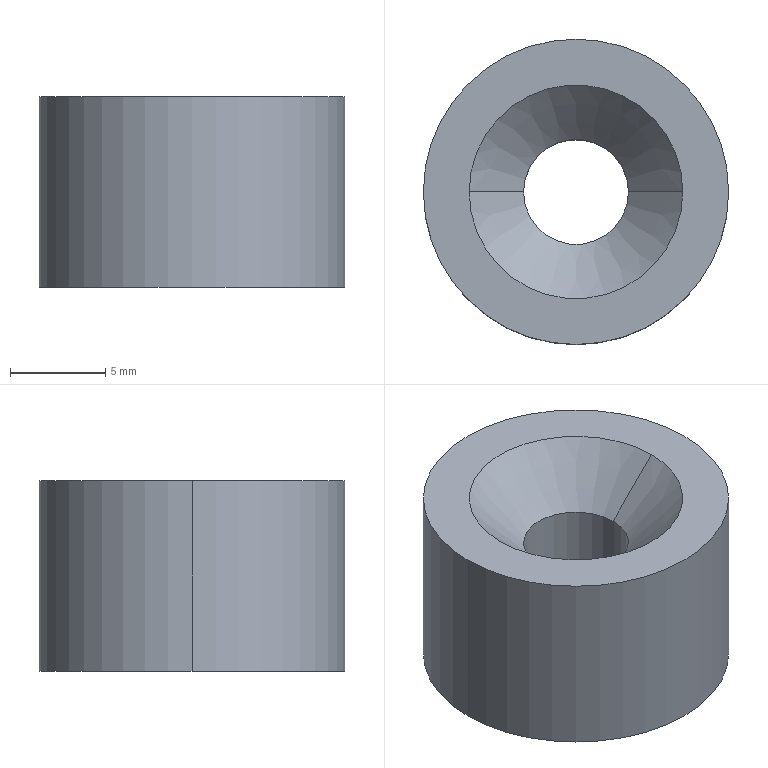Part | STEP file | Clamping Pad | 1 solid | 8 faces | box 16 x 16 x 10 mm | volume 1679 mm3 | cylinder 4 | cone 2 | plane 2 | commonest cylinder face diameters 5.5 x2 16 x2
STEP:
#1=CARTESIAN_POINT('',(0.,0.,0.));
#2=DIRECTION('',(0.,0.,1.));
#3=DIRECTION('',(1.,0.,0.));
#4=AXIS2_PLACEMENT_3D('',#1,#2,#3);
#5=CARTESIAN_POINT('',(2.75,0.,7.15));
#6=VERTEX_POINT('',#5);
#7=CARTESIAN_POINT('',(5.6,0.,10.));
#8=VERTEX_POINT('',#7);
#9=CARTESIAN_POINT('',(5.6,0.,10.));
#10=DIRECTION('',(0.7071,0.,0.7071));
#11=VECTOR('',#10,1.);
#12=LINE('',#9,#11);
#13=CARTESIAN_POINT('',(0.,0.,10.));
#14=DIRECTION('',(0.,0.,1.));
#15=DIRECTION('',(1.,0.,0.));
#16=AXIS2_PLACEMENT_3D('',#13,#14,#15);
#17=CONICAL_SURFACE('',#16,5.6,0.7854);
#18=CARTESIAN_POINT('',(6.283,0.));
#19=DIRECTION('',(0.,1.));
#20=VECTOR('',#19,1.);
#21=LINE('',#18,#20);
#22=(GEOMETRIC_REPRESENTATION_CONTEXT(2)PARAMETRIC_REPRESENTATION_CONTEXT()REPRESENTATION_CONTEXT('',''));
#23=DEFINITIONAL_REPRESENTATION('',(#21),#22);
#24=PCURVE('',#17,#23);
#25=CARTESIAN_POINT('',(0.,0.,10.));
#26=DIRECTION('',(0.,0.,1.));
#27=DIRECTION('',(1.,0.,0.));
#28=AXIS2_PLACEMENT_3D('',#25,#26,#27);
#29=CONICAL_SURFACE('',#28,5.6,0.7854);
#30=CARTESIAN_POINT('',(0.,0.));
#31=DIRECTION('',(0.,1.));
#32=VECTOR('',#31,1.);
#33=LINE('',#30,#32);
#34=(GEOMETRIC_REPRESENTATION_CONTEXT(2)PARAMETRIC_REPRESENTATION_CONTEXT()REPRESENTATION_CONTEXT('',''));
#35=DEFINITIONAL_REPRESENTATION('',(#33),#34);
#36=PCURVE('',#29,#35);
#37=SURFACE_CURVE('',#12,(#24,#36),.PCURVE_S1.);
#38=EDGE_CURVE('',#6,#8,#37,.T.);
#39=ORIENTED_EDGE('',*,*,#38,.T.);
#40=CARTESIAN_POINT('',(-5.6,0.,10.));
#41=VERTEX_POINT('',#40);
#42=CARTESIAN_POINT('',(0.,0.,10.));
#43=DIRECTION('',(0.,0.,1.));
#44=DIRECTION('',(1.,0.,0.));
#45=AXIS2_PLACEMENT_3D('',#42,#43,#44);
#46=CIRCLE('',#45,5.6);
#47=CARTESIAN_POINT('',(0.,0.));
#48=DIRECTION('',(1.,0.));
#49=VECTOR('',#48,1.);
#50=LINE('',#47,#49);
#51=(GEOMETRIC_REPRESENTATION_CONTEXT(2)PARAMETRIC_REPRESENTATION_CONTEXT()REPRESENTATION_CONTEXT('',''));
#52=DEFINITIONAL_REPRESENTATION('',(#50),#51);
#53=PCURVE('',#17,#52);
#54=CARTESIAN_POINT('',(0.,0.,10.));
#55=DIRECTION('',(0.,0.,1.));
#56=DIRECTION('',(1.,0.,0.));
#57=AXIS2_PLACEMENT_3D('',#54,#55,#56);
#58=PLANE('',#57);
#59=CARTESIAN_POINT('',(0.,0.));
#60=DIRECTION('',(1.,0.));
#61=AXIS2_PLACEMENT_2D('',#59,#60);
#62=CIRCLE('',#61,5.6);
#63=(GEOMETRIC_REPRESENTATION_CONTEXT(2)PARAMETRIC_REPRESENTATION_CONTEXT()REPRESENTATION_CONTEXT('',''));
#64=DEFINITIONAL_REPRESENTATION('',(#62),#63);
#65=PCURVE('',#58,#64);
#66=SURFACE_CURVE('',#46,(#53,#65),.PCURVE_S1.);
#67=EDGE_CURVE('',#41,#8,#66,.T.);
#68=ORIENTED_EDGE('',*,*,#67,.F.);
#69=CARTESIAN_POINT('',(-2.75,0.,7.15));
#70=VERTEX_POINT('',#69);
#71=CARTESIAN_POINT('',(-5.6,0.,10.));
#72=DIRECTION('',(-0.7071,0.,0.7071));
#73=VECTOR('',#72,1.);
#74=LINE('',#71,#73);
#75=CARTESIAN_POINT('',(3.142,0.));
#76=DIRECTION('',(0.,1.));
#77=VECTOR('',#76,1.);
#78=LINE('',#75,#77);
#79=(GEOMETRIC_REPRESENTATION_CONTEXT(2)PARAMETRIC_REPRESENTATION_CONTEXT()REPRESENTATION_CONTEXT('',''));
#80=DEFINITIONAL_REPRESENTATION('',(#78),#79);
#81=PCURVE('',#17,#80);
#82=CARTESIAN_POINT('',(3.142,0.));
#83=DIRECTION('',(0.,1.));
#84=VECTOR('',#83,1.);
#85=LINE('',#82,#84);
#86=(GEOMETRIC_REPRESENTATION_CONTEXT(2)PARAMETRIC_REPRESENTATION_CONTEXT()REPRESENTATION_CONTEXT('',''));
#87=DEFINITIONAL_REPRESENTATION('',(#85),#86);
#88=PCURVE('',#29,#87);
#89=SURFACE_CURVE('',#74,(#81,#88),.PCURVE_S1.);
#90=EDGE_CURVE('',#70,#41,#89,.T.);
#91=ORIENTED_EDGE('',*,*,#90,.F.);
#92=CARTESIAN_POINT('',(0.,0.,7.15));
#93=DIRECTION('',(0.,0.,1.));
#94=DIRECTION('',(1.,0.,0.));
#95=AXIS2_PLACEMENT_3D('',#92,#93,#94);
#96=CIRCLE('',#95,2.75);
#97=CARTESIAN_POINT('',(0.,-2.85));
#98=DIRECTION('',(1.,0.));
#99=VECTOR('',#98,1.);
#100=LINE('',#97,#99);
#101=(GEOMETRIC_REPRESENTATION_CONTEXT(2)PARAMETRIC_REPRESENTATION_CONTEXT()REPRESENTATION_CONTEXT('',''));
#102=DEFINITIONAL_REPRESENTATION('',(#100),#101);
#103=PCURVE('',#17,#102);
#104=CARTESIAN_POINT('',(0.,0.,10.));
#105=DIRECTION('',(0.,0.,1.));
#106=DIRECTION('',(1.,0.,0.));
#107=AXIS2_PLACEMENT_3D('',#104,#105,#106);
#108=CYLINDRICAL_SURFACE('',#107,2.75);
#109=CARTESIAN_POINT('',(0.,-2.85));
#110=DIRECTION('',(1.,0.));
#111=VECTOR('',#110,1.);
#112=LINE('',#109,#111);
#113=(GEOMETRIC_REPRESENTATION_CONTEXT(2)PARAMETRIC_REPRESENTATION_CONTEXT()REPRESENTATION_CONTEXT('',''));
#114=DEFINITIONAL_REPRESENTATION('',(#112),#113);
#115=PCURVE('',#108,#114);
#116=SURFACE_CURVE('',#96,(#103,#115),.PCURVE_S1.);
#117=EDGE_CURVE('',#70,#6,#116,.T.);
#118=ORIENTED_EDGE('',*,*,#117,.T.);
#119=EDGE_LOOP('',(#39,#68,#91,#118));
#120=FACE_BOUND('',#119,.F.);
#121=ADVANCED_FACE('',(#120),#17,.F.);
#122=CARTESIAN_POINT('',(2.75,0.,0.));
#123=VERTEX_POINT('',#122);
#124=CARTESIAN_POINT('',(2.75,0.,10.));
#125=DIRECTION('',(0.,0.,1.));
#126=VECTOR('',#125,1.);
#127=LINE('',#124,#126);
#128=CARTESIAN_POINT('',(6.283,0.));
#129=DIRECTION('',(0.,1.));
#130=VECTOR('',#129,1.);
#131=LINE('',#128,#130);
#132=(GEOMETRIC_REPRESENTATION_CONTEXT(2)PARAMETRIC_REPRESENTATION_CONTEXT()REPRESENTATION_CONTEXT('',''));
#133=DEFINITIONAL_REPRESENTATION('',(#131),#132);
#134=PCURVE('',#108,#133);
#135=CARTESIAN_POINT('',(0.,0.,10.));
#136=DIRECTION('',(0.,0.,1.));
#137=DIRECTION('',(1.,0.,0.));
#138=AXIS2_PLACEMENT_3D('',#135,#136,#137);
#139=CYLINDRICAL_SURFACE('',#138,2.75);
#140=CARTESIAN_POINT('',(0.,0.));
#141=DIRECTION('',(0.,1.));
#142=VECTOR('',#141,1.);
#143=LINE('',#140,#142);
#144=(GEOMETRIC_REPRESENTATION_CONTEXT(2)PARAMETRIC_REPRESENTATION_CONTEXT()REPRESENTATION_CONTEXT('',''));
#145=DEFINITIONAL_REPRESENTATION('',(#143),#144);
#146=PCURVE('',#139,#145);
#147=SURFACE_CURVE('',#127,(#134,#146),.PCURVE_S1.);
#148=EDGE_CURVE('',#123,#6,#147,.T.);
#149=ORIENTED_EDGE('',*,*,#148,.T.);
#150=ORIENTED_EDGE('',*,*,#117,.F.);
#151=CARTESIAN_POINT('',(-2.75,0.,0.));
#152=VERTEX_POINT('',#151);
#153=CARTESIAN_POINT('',(-2.75,0.,10.));
#154=DIRECTION('',(0.,0.,1.));
#155=VECTOR('',#154,1.);
#156=LINE('',#153,#155);
#157=CARTESIAN_POINT('',(3.142,0.));
#158=DIRECTION('',(0.,1.));
#159=VECTOR('',#158,1.);
#160=LINE('',#157,#159);
#161=(GEOMETRIC_REPRESENTATION_CONTEXT(2)PARAMETRIC_REPRESENTATION_CONTEXT()REPRESENTATION_CONTEXT('',''));
#162=DEFINITIONAL_REPRESENTATION('',(#160),#161);
#163=PCURVE('',#108,#162);
#164=CARTESIAN_POINT('',(3.142,0.));
#165=DIRECTION('',(0.,1.));
#166=VECTOR('',#165,1.);
#167=LINE('',#164,#166);
#168=(GEOMETRIC_REPRESENTATION_CONTEXT(2)PARAMETRIC_REPRESENTATION_CONTEXT()REPRESENTATION_CONTEXT('',''));
#169=DEFINITIONAL_REPRESENTATION('',(#167),#168);
#170=PCURVE('',#139,#169);
#171=SURFACE_CURVE('',#156,(#163,#170),.PCURVE_S1.);
#172=EDGE_CURVE('',#152,#70,#171,.T.);
#173=ORIENTED_EDGE('',*,*,#172,.F.);
#174=CARTESIAN_POINT('',(0.,0.,0.));
#175=DIRECTION('',(0.,0.,1.));
#176=DIRECTION('',(1.,0.,0.));
#177=AXIS2_PLACEMENT_3D('',#174,#175,#176);
#178=CIRCLE('',#177,2.75);
#179=CARTESIAN_POINT('',(0.,-10.));
#180=DIRECTION('',(1.,0.));
#181=VECTOR('',#180,1.);
#182=LINE('',#179,#181);
#183=(GEOMETRIC_REPRESENTATION_CONTEXT(2)PARAMETRIC_REPRESENTATION_CONTEXT()REPRESENTATION_CONTEXT('',''));
#184=DEFINITIONAL_REPRESENTATION('',(#182),#183);
#185=PCURVE('',#108,#184);
#186=CARTESIAN_POINT('',(0.,0.,0.));
#187=DIRECTION('',(0.,0.,1.));
#188=DIRECTION('',(1.,0.,0.));
#189=AXIS2_PLACEMENT_3D('',#186,#187,#188);
#190=PLANE('',#189);
#191=CARTESIAN_POINT('',(0.,0.));
#192=DIRECTION('',(1.,0.));
#193=AXIS2_PLACEMENT_2D('',#191,#192);
#194=CIRCLE('',#193,2.75);
#195=(GEOMETRIC_REPRESENTATION_CONTEXT(2)PARAMETRIC_REPRESENTATION_CONTEXT()REPRESENTATION_CONTEXT('',''));
#196=DEFINITIONAL_REPRESENTATION('',(#194),#195);
#197=PCURVE('',#190,#196);
#198=SURFACE_CURVE('',#178,(#185,#197),.PCURVE_S1.);
#199=EDGE_CURVE('',#152,#123,#198,.T.);
#200=ORIENTED_EDGE('',*,*,#199,.T.);
#201=EDGE_LOOP('',(#149,#150,#173,#200));
#202=FACE_BOUND('',#201,.F.);
#203=ADVANCED_FACE('',(#202),#108,.F.);
#204=CARTESIAN_POINT('',(8.,0.,10.));
#205=VERTEX_POINT('',#204);
#206=CARTESIAN_POINT('',(-8.,0.,10.));
#207=VERTEX_POINT('',#206);
#208=CARTESIAN_POINT('',(0.,0.,10.));
#209=DIRECTION('',(0.,0.,1.));
#210=DIRECTION('',(1.,0.,0.));
#211=AXIS2_PLACEMENT_3D('',#208,#209,#210);
#212=CIRCLE('',#211,8.);
#213=CARTESIAN_POINT('',(0.,0.,10.));
#214=DIRECTION('',(0.,0.,-1.));
#215=DIRECTION('',(-1.,0.,0.));
#216=AXIS2_PLACEMENT_3D('',#213,#214,#215);
#217=CYLINDRICAL_SURFACE('',#216,8.);
#218=CARTESIAN_POINT('',(3.142,0.));
#219=DIRECTION('',(-1.,0.));
#220=VECTOR('',#219,1.);
#221=LINE('',#218,#220);
#222=(GEOMETRIC_REPRESENTATION_CONTEXT(2)PARAMETRIC_REPRESENTATION_CONTEXT()REPRESENTATION_CONTEXT('',''));
#223=DEFINITIONAL_REPRESENTATION('',(#221),#222);
#224=PCURVE('',#217,#223);
#225=CARTESIAN_POINT('',(0.,0.));
#226=DIRECTION('',(1.,0.));
#227=AXIS2_PLACEMENT_2D('',#225,#226);
#228=CIRCLE('',#227,8.);
#229=(GEOMETRIC_REPRESENTATION_CONTEXT(2)PARAMETRIC_REPRESENTATION_CONTEXT()REPRESENTATION_CONTEXT('',''));
#230=DEFINITIONAL_REPRESENTATION('',(#228),#229);
#231=PCURVE('',#58,#230);
#232=SURFACE_CURVE('',#212,(#224,#231),.PCURVE_S1.);
#233=EDGE_CURVE('',#205,#207,#232,.T.);
#234=ORIENTED_EDGE('',*,*,#233,.F.);
#235=CARTESIAN_POINT('',(8.,0.,0.));
#236=VERTEX_POINT('',#235);
#237=CARTESIAN_POINT('',(8.,0.,10.));
#238=DIRECTION('',(0.,0.,-1.));
#239=VECTOR('',#238,1.);
#240=LINE('',#237,#239);
#241=CARTESIAN_POINT('',(3.142,0.));
#242=DIRECTION('',(0.,1.));
#243=VECTOR('',#242,1.);
#244=LINE('',#241,#243);
#245=(GEOMETRIC_REPRESENTATION_CONTEXT(2)PARAMETRIC_REPRESENTATION_CONTEXT()REPRESENTATION_CONTEXT('',''));
#246=DEFINITIONAL_REPRESENTATION('',(#244),#245);
#247=PCURVE('',#217,#246);
#248=CARTESIAN_POINT('',(0.,0.,10.));
#249=DIRECTION('',(0.,0.,-1.));
#250=DIRECTION('',(-1.,0.,0.));
#251=AXIS2_PLACEMENT_3D('',#248,#249,#250);
#252=CYLINDRICAL_SURFACE('',#251,8.);
#253=CARTESIAN_POINT('',(3.142,0.));
#254=DIRECTION('',(0.,1.));
#255=VECTOR('',#254,1.);
#256=LINE('',#253,#255);
#257=(GEOMETRIC_REPRESENTATION_CONTEXT(2)PARAMETRIC_REPRESENTATION_CONTEXT()REPRESENTATION_CONTEXT('',''));
#258=DEFINITIONAL_REPRESENTATION('',(#256),#257);
#259=PCURVE('',#252,#258);
#260=SURFACE_CURVE('',#240,(#247,#259),.PCURVE_S1.);
#261=EDGE_CURVE('',#205,#236,#260,.T.);
#262=ORIENTED_EDGE('',*,*,#261,.T.);
#263=CARTESIAN_POINT('',(-8.,0.,0.));
#264=VERTEX_POINT('',#263);
#265=CARTESIAN_POINT('',(0.,0.,0.));
#266=DIRECTION('',(0.,0.,1.));
#267=DIRECTION('',(1.,0.,0.));
#268=AXIS2_PLACEMENT_3D('',#265,#266,#267);
#269=CIRCLE('',#268,8.);
#270=CARTESIAN_POINT('',(3.142,10.));
#271=DIRECTION('',(-1.,0.));
#272=VECTOR('',#271,1.);
#273=LINE('',#270,#272);
#274=(GEOMETRIC_REPRESENTATION_CONTEXT(2)PARAMETRIC_REPRESENTATION_CONTEXT()REPRESENTATION_CONTEXT('',''));
#275=DEFINITIONAL_REPRESENTATION('',(#273),#274);
#276=PCURVE('',#217,#275);
#277=CARTESIAN_POINT('',(0.,0.));
#278=DIRECTION('',(1.,0.));
#279=AXIS2_PLACEMENT_2D('',#277,#278);
#280=CIRCLE('',#279,8.);
#281=(GEOMETRIC_REPRESENTATION_CONTEXT(2)PARAMETRIC_REPRESENTATION_CONTEXT()REPRESENTATION_CONTEXT('',''));
#282=DEFINITIONAL_REPRESENTATION('',(#280),#281);
#283=PCURVE('',#190,#282);
#284=SURFACE_CURVE('',#269,(#276,#283),.PCURVE_S1.);
#285=EDGE_CURVE('',#236,#264,#284,.T.);
#286=ORIENTED_EDGE('',*,*,#285,.T.);
#287=CARTESIAN_POINT('',(-8.,0.,10.));
#288=DIRECTION('',(0.,0.,-1.));
#289=VECTOR('',#288,1.);
#290=LINE('',#287,#289);
#291=CARTESIAN_POINT('',(0.,0.));
#292=DIRECTION('',(0.,1.));
#293=VECTOR('',#292,1.);
#294=LINE('',#291,#293);
#295=(GEOMETRIC_REPRESENTATION_CONTEXT(2)PARAMETRIC_REPRESENTATION_CONTEXT()REPRESENTATION_CONTEXT('',''));
#296=DEFINITIONAL_REPRESENTATION('',(#294),#295);
#297=PCURVE('',#217,#296);
#298=CARTESIAN_POINT('',(6.283,0.));
#299=DIRECTION('',(0.,1.));
#300=VECTOR('',#299,1.);
#301=LINE('',#298,#300);
#302=(GEOMETRIC_REPRESENTATION_CONTEXT(2)PARAMETRIC_REPRESENTATION_CONTEXT()REPRESENTATION_CONTEXT('',''));
#303=DEFINITIONAL_REPRESENTATION('',(#301),#302);
#304=PCURVE('',#252,#303);
#305=SURFACE_CURVE('',#290,(#297,#304),.PCURVE_S1.);
#306=EDGE_CURVE('',#207,#264,#305,.T.);
#307=ORIENTED_EDGE('',*,*,#306,.F.);
#308=EDGE_LOOP('',(#234,#262,#286,#307));
#309=FACE_BOUND('',#308,.T.);
#310=ADVANCED_FACE('',(#309),#217,.T.);
#311=ORIENTED_EDGE('',*,*,#261,.F.);
#312=CARTESIAN_POINT('',(0.,0.,10.));
#313=DIRECTION('',(0.,0.,1.));
#314=DIRECTION('',(1.,0.,0.));
#315=AXIS2_PLACEMENT_3D('',#312,#313,#314);
#316=CIRCLE('',#315,8.);
#317=CARTESIAN_POINT('',(9.425,0.));
#318=DIRECTION('',(-1.,0.));
#319=VECTOR('',#318,1.);
#320=LINE('',#317,#319);
#321=(GEOMETRIC_REPRESENTATION_CONTEXT(2)PARAMETRIC_REPRESENTATION_CONTEXT()REPRESENTATION_CONTEXT('',''));
#322=DEFINITIONAL_REPRESENTATION('',(#320),#321);
#323=PCURVE('',#252,#322);
#324=CARTESIAN_POINT('',(0.,0.));
#325=DIRECTION('',(1.,0.));
#326=AXIS2_PLACEMENT_2D('',#324,#325);
#327=CIRCLE('',#326,8.);
#328=(GEOMETRIC_REPRESENTATION_CONTEXT(2)PARAMETRIC_REPRESENTATION_CONTEXT()REPRESENTATION_CONTEXT('',''));
#329=DEFINITIONAL_REPRESENTATION('',(#327),#328);
#330=PCURVE('',#58,#329);
#331=SURFACE_CURVE('',#316,(#323,#330),.PCURVE_S1.);
#332=EDGE_CURVE('',#207,#205,#331,.T.);
#333=ORIENTED_EDGE('',*,*,#332,.F.);
#334=ORIENTED_EDGE('',*,*,#306,.T.);
#335=CARTESIAN_POINT('',(0.,0.,0.));
#336=DIRECTION('',(0.,0.,1.));
#337=DIRECTION('',(1.,0.,0.));
#338=AXIS2_PLACEMENT_3D('',#335,#336,#337);
#339=CIRCLE('',#338,8.);
#340=CARTESIAN_POINT('',(9.425,10.));
#341=DIRECTION('',(-1.,0.));
#342=VECTOR('',#341,1.);
#343=LINE('',#340,#342);
#344=(GEOMETRIC_REPRESENTATION_CONTEXT(2)PARAMETRIC_REPRESENTATION_CONTEXT()REPRESENTATION_CONTEXT('',''));
#345=DEFINITIONAL_REPRESENTATION('',(#343),#344);
#346=PCURVE('',#252,#345);
#347=CARTESIAN_POINT('',(0.,0.));
#348=DIRECTION('',(1.,0.));
#349=AXIS2_PLACEMENT_2D('',#347,#348);
#350=CIRCLE('',#349,8.);
#351=(GEOMETRIC_REPRESENTATION_CONTEXT(2)PARAMETRIC_REPRESENTATION_CONTEXT()REPRESENTATION_CONTEXT('',''));
#352=DEFINITIONAL_REPRESENTATION('',(#350),#351);
#353=PCURVE('',#190,#352);
#354=SURFACE_CURVE('',#339,(#346,#353),.PCURVE_S1.);
#355=EDGE_CURVE('',#264,#236,#354,.T.);
#356=ORIENTED_EDGE('',*,*,#355,.T.);
#357=EDGE_LOOP('',(#311,#333,#334,#356));
#358=FACE_BOUND('',#357,.T.);
#359=ADVANCED_FACE('',(#358),#252,.T.);
#360=CARTESIAN_POINT('',(0.,0.,10.));
#361=DIRECTION('',(0.,0.,1.));
#362=DIRECTION('',(1.,0.,0.));
#363=AXIS2_PLACEMENT_3D('',#360,#361,#362);
#364=CIRCLE('',#363,5.6);
#365=CARTESIAN_POINT('',(0.,0.));
#366=DIRECTION('',(1.,0.));
#367=AXIS2_PLACEMENT_2D('',#365,#366);
#368=CIRCLE('',#367,5.6);
#369=(GEOMETRIC_REPRESENTATION_CONTEXT(2)PARAMETRIC_REPRESENTATION_CONTEXT()REPRESENTATION_CONTEXT('',''));
#370=DEFINITIONAL_REPRESENTATION('',(#368),#369);
#371=PCURVE('',#58,#370);
#372=CARTESIAN_POINT('',(0.,0.));
#373=DIRECTION('',(1.,0.));
#374=VECTOR('',#373,1.);
#375=LINE('',#372,#374);
#376=(GEOMETRIC_REPRESENTATION_CONTEXT(2)PARAMETRIC_REPRESENTATION_CONTEXT()REPRESENTATION_CONTEXT('',''));
#377=DEFINITIONAL_REPRESENTATION('',(#375),#376);
#378=PCURVE('',#29,#377);
#379=SURFACE_CURVE('',#364,(#371,#378),.PCURVE_S1.);
#380=EDGE_CURVE('',#8,#41,#379,.T.);
#381=ORIENTED_EDGE('',*,*,#380,.F.);
#382=ORIENTED_EDGE('',*,*,#67,.F.);
#383=EDGE_LOOP('',(#381,#382));
#384=FACE_BOUND('',#383,.T.);
#385=ORIENTED_EDGE('',*,*,#332,.T.);
#386=ORIENTED_EDGE('',*,*,#233,.T.);
#387=EDGE_LOOP('',(#385,#386));
#388=FACE_BOUND('',#387,.T.);
#389=ADVANCED_FACE('',(#384,#388),#58,.T.);
#390=CARTESIAN_POINT('',(0.,0.,0.));
#391=DIRECTION('',(0.,0.,1.));
#392=DIRECTION('',(1.,0.,0.));
#393=AXIS2_PLACEMENT_3D('',#390,#391,#392);
#394=CIRCLE('',#393,2.75);
#395=CARTESIAN_POINT('',(0.,0.));
#396=DIRECTION('',(1.,0.));
#397=AXIS2_PLACEMENT_2D('',#395,#396);
#398=CIRCLE('',#397,2.75);
#399=(GEOMETRIC_REPRESENTATION_CONTEXT(2)PARAMETRIC_REPRESENTATION_CONTEXT()REPRESENTATION_CONTEXT('',''));
#400=DEFINITIONAL_REPRESENTATION('',(#398),#399);
#401=PCURVE('',#190,#400);
#402=CARTESIAN_POINT('',(0.,-10.));
#403=DIRECTION('',(1.,0.));
#404=VECTOR('',#403,1.);
#405=LINE('',#402,#404);
#406=(GEOMETRIC_REPRESENTATION_CONTEXT(2)PARAMETRIC_REPRESENTATION_CONTEXT()REPRESENTATION_CONTEXT('',''));
#407=DEFINITIONAL_REPRESENTATION('',(#405),#406);
#408=PCURVE('',#139,#407);
#409=SURFACE_CURVE('',#394,(#401,#408),.PCURVE_S1.);
#410=EDGE_CURVE('',#123,#152,#409,.T.);
#411=ORIENTED_EDGE('',*,*,#410,.T.);
#412=ORIENTED_EDGE('',*,*,#199,.T.);
#413=EDGE_LOOP('',(#411,#412));
#414=FACE_BOUND('',#413,.T.);
#415=ORIENTED_EDGE('',*,*,#355,.F.);
#416=ORIENTED_EDGE('',*,*,#285,.F.);
#417=EDGE_LOOP('',(#415,#416));
#418=FACE_BOUND('',#417,.T.);
#419=ADVANCED_FACE('',(#414,#418),#190,.F.);
#420=CARTESIAN_POINT('',(0.,0.,7.15));
#421=DIRECTION('',(0.,0.,1.));
#422=DIRECTION('',(1.,0.,0.));
#423=AXIS2_PLACEMENT_3D('',#420,#421,#422);
#424=CIRCLE('',#423,2.75);
#425=CARTESIAN_POINT('',(0.,-2.85));
#426=DIRECTION('',(1.,0.));
#427=VECTOR('',#426,1.);
#428=LINE('',#425,#427);
#429=(GEOMETRIC_REPRESENTATION_CONTEXT(2)PARAMETRIC_REPRESENTATION_CONTEXT()REPRESENTATION_CONTEXT('',''));
#430=DEFINITIONAL_REPRESENTATION('',(#428),#429);
#431=PCURVE('',#139,#430);
#432=CARTESIAN_POINT('',(0.,-2.85));
#433=DIRECTION('',(1.,0.));
#434=VECTOR('',#433,1.);
#435=LINE('',#432,#434);
#436=(GEOMETRIC_REPRESENTATION_CONTEXT(2)PARAMETRIC_REPRESENTATION_CONTEXT()REPRESENTATION_CONTEXT('',''));
#437=DEFINITIONAL_REPRESENTATION('',(#435),#436);
#438=PCURVE('',#29,#437);
#439=SURFACE_CURVE('',#424,(#431,#438),.PCURVE_S1.);
#440=EDGE_CURVE('',#6,#70,#439,.T.);
#441=ORIENTED_EDGE('',*,*,#440,.F.);
#442=ORIENTED_EDGE('',*,*,#148,.F.);
#443=ORIENTED_EDGE('',*,*,#410,.T.);
#444=ORIENTED_EDGE('',*,*,#172,.T.);
#445=EDGE_LOOP('',(#441,#442,#443,#444));
#446=FACE_BOUND('',#445,.F.);
#447=ADVANCED_FACE('',(#446),#139,.F.);
#448=ORIENTED_EDGE('',*,*,#380,.F.);
#449=ORIENTED_EDGE('',*,*,#38,.F.);
#450=ORIENTED_EDGE('',*,*,#440,.T.);
#451=ORIENTED_EDGE('',*,*,#90,.T.);
#452=EDGE_LOOP('',(#448,#449,#450,#451));
#453=FACE_BOUND('',#452,.F.);
#454=ADVANCED_FACE('',(#453),#29,.F.);
#455=CLOSED_SHELL('',(#121,#203,#310,#359,#389,#419,#447,#454));
#456=MANIFOLD_SOLID_BREP('',#455);
#457=(LENGTH_UNIT()NAMED_UNIT(*)SI_UNIT(.MILLI.,.METRE.));
#458=UNCERTAINTY_MEASURE_WITH_UNIT(LENGTH_MEASURE(0.0000001),#457,'','');
#459=(NAMED_UNIT(*)PLANE_ANGLE_UNIT()SI_UNIT($,.RADIAN.));
#460=(NAMED_UNIT(*)SI_UNIT($,.STERADIAN.)SOLID_ANGLE_UNIT());
#461=(GEOMETRIC_REPRESENTATION_CONTEXT(3)GLOBAL_UNCERTAINTY_ASSIGNED_CONTEXT((#458))GLOBAL_UNIT_ASSIGNED_CONTEXT((#457,#459,#460))REPRESENTATION_CONTEXT('',''));
#462=ADVANCED_BREP_SHAPE_REPRESENTATION('',(#4,#456),#461);